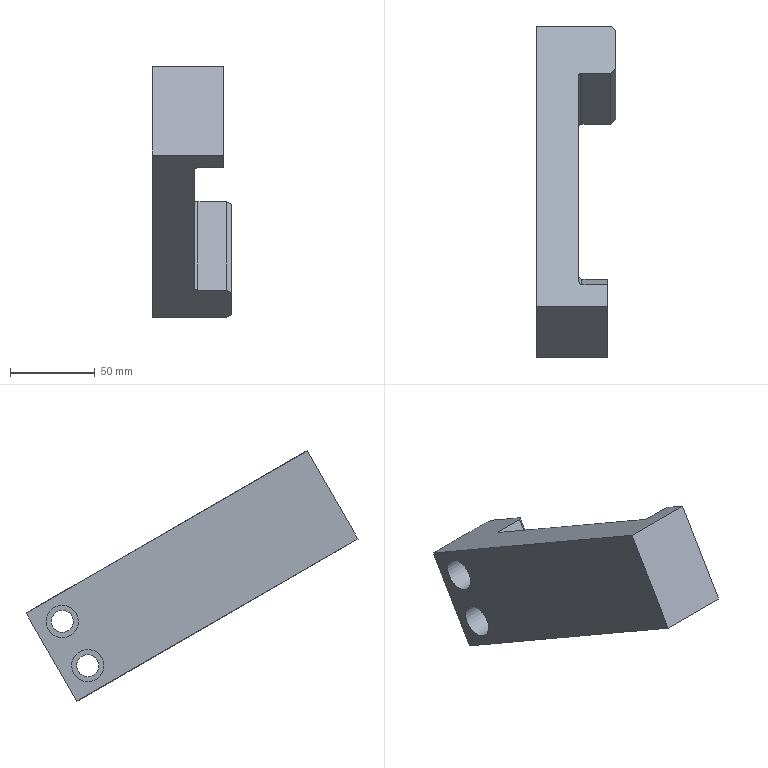Part | NX | features MAIN_BODY 2 | 1 solid | 28 faces | box 47 x 195.411 x 147.462 mm | volume 335091 mm3 | plane 16 | cylinder 10 | spline 2 | commonest cylinder face diameters 4 x4 10 x2 13 x2 19 x2
STEP:
#1=CARTESIAN_POINT('',(-607.,713.604,-62.591));
#2=VERTEX_POINT('',#1);
#3=CARTESIAN_POINT('',(-607.,721.831,-67.341));
#4=DIRECTION('',(-1.,0.,0.));
#5=DIRECTION('',(0.,-0.866,0.5));
#6=AXIS2_PLACEMENT_3D('',#3,#4,#5);
#7=CIRCLE('',#6,9.5);
#8=EDGE_CURVE('',#2,#2,#7,.T.);
#9=ORIENTED_EDGE('',*,*,#8,.F.);
#10=EDGE_LOOP('',(#9));
#11=FACE_BOUND('',#10,.T.);
#12=CARTESIAN_POINT('',(-607.,743.188,-62.351));
#13=VERTEX_POINT('',#12);
#14=CARTESIAN_POINT('',(-607.,577.777,33.149));
#15=VERTEX_POINT('',#14);
#16=CARTESIAN_POINT('',(-607.,743.188,-62.351));
#17=DIRECTION('',(0.,-0.866,0.5));
#18=VECTOR('',#17,1000.);
#19=LINE('',#16,#18);
#20=EDGE_CURVE('',#13,#15,#19,.T.);
#21=ORIENTED_EDGE('',*,*,#20,.F.);
#22=CARTESIAN_POINT('',(-607.,713.188,-114.312));
#23=VERTEX_POINT('',#22);
#24=CARTESIAN_POINT('',(-607.,713.188,-114.312));
#25=DIRECTION('',(0.,0.5,0.866));
#26=VECTOR('',#25,1000.);
#27=LINE('',#24,#26);
#28=EDGE_CURVE('',#23,#13,#27,.T.);
#29=ORIENTED_EDGE('',*,*,#28,.F.);
#30=CARTESIAN_POINT('',(-607.,547.777,-18.812));
#31=VERTEX_POINT('',#30);
#32=CARTESIAN_POINT('',(-607.,547.777,-18.812));
#33=DIRECTION('',(0.,0.866,-0.5));
#34=VECTOR('',#33,1000.);
#35=LINE('',#32,#34);
#36=EDGE_CURVE('',#31,#23,#35,.T.);
#37=ORIENTED_EDGE('',*,*,#36,.F.);
#38=CARTESIAN_POINT('',(-607.,577.777,33.149));
#39=DIRECTION('',(0.,-0.5,-0.866));
#40=VECTOR('',#39,1000.);
#41=LINE('',#38,#40);
#42=EDGE_CURVE('',#15,#31,#41,.T.);
#43=ORIENTED_EDGE('',*,*,#42,.F.);
#44=EDGE_LOOP('',(#21,#29,#37,#43));
#45=FACE_BOUND('',#44,.T.);
#46=CARTESIAN_POINT('',(-607.,698.604,-88.572));
#47=VERTEX_POINT('',#46);
#48=CARTESIAN_POINT('',(-607.,706.831,-93.322));
#49=DIRECTION('',(-1.,0.,0.));
#50=DIRECTION('',(0.,-0.866,0.5));
#51=AXIS2_PLACEMENT_3D('',#48,#49,#50);
#52=CIRCLE('',#51,9.5);
#53=EDGE_CURVE('',#47,#47,#52,.T.);
#54=ORIENTED_EDGE('',*,*,#53,.F.);
#55=EDGE_LOOP('',(#54));
#56=FACE_BOUND('',#55,.T.);
#57=CARTESIAN_POINT('',(-607.,743.188,-62.351));
#58=DIRECTION('',(-1.,0.,0.));
#59=DIRECTION('',(0.,0.866,-0.5));
#60=AXIS2_PLACEMENT_3D('',#57,#58,#59);
#61=PLANE('',#60);
#62=ADVANCED_FACE('',(#11,#45,#56),#61,.T.);
#63=CARTESIAN_POINT('',(-560.,716.202,-64.091));
#64=VERTEX_POINT('',#63);
#65=CARTESIAN_POINT('',(-560.,721.831,-67.341));
#66=DIRECTION('',(-1.,0.,0.));
#67=DIRECTION('',(0.,-0.866,0.5));
#68=AXIS2_PLACEMENT_3D('',#65,#66,#67);
#69=CIRCLE('',#68,6.5);
#70=EDGE_CURVE('',#64,#64,#69,.T.);
#71=ORIENTED_EDGE('',*,*,#70,.T.);
#72=EDGE_LOOP('',(#71));
#73=FACE_BOUND('',#72,.T.);
#74=CARTESIAN_POINT('',(-560.,688.073,-99.812));
#75=VERTEX_POINT('',#74);
#76=CARTESIAN_POINT('',(-560.,710.589,-112.812));
#77=VERTEX_POINT('',#76);
#78=CARTESIAN_POINT('',(-560.,685.475,-98.312));
#79=DIRECTION('',(0.,0.866,-0.5));
#80=VECTOR('',#79,1000.);
#81=LINE('',#78,#80);
#82=EDGE_CURVE('',#75,#77,#81,.T.);
#83=ORIENTED_EDGE('',*,*,#82,.T.);
#84=CARTESIAN_POINT('',(-560.,740.589,-60.851));
#85=VERTEX_POINT('',#84);
#86=CARTESIAN_POINT('',(-560.,710.589,-112.812));
#87=DIRECTION('',(0.,-0.5,-0.866));
#88=VECTOR('',#87,1000.);
#89=LINE('',#86,#88);
#90=EDGE_CURVE('',#85,#77,#89,.T.);
#91=ORIENTED_EDGE('',*,*,#90,.F.);
#92=CARTESIAN_POINT('',(-560.,718.073,-47.851));
#93=VERTEX_POINT('',#92);
#94=CARTESIAN_POINT('',(-560.,743.188,-62.351));
#95=DIRECTION('',(0.,-0.866,0.5));
#96=VECTOR('',#95,1000.);
#97=LINE('',#94,#96);
#98=EDGE_CURVE('',#85,#93,#97,.T.);
#99=ORIENTED_EDGE('',*,*,#98,.T.);
#100=CARTESIAN_POINT('',(-560.,718.073,-47.851));
#101=DIRECTION('',(0.,0.5,0.866));
#102=VECTOR('',#101,1000.);
#103=LINE('',#100,#102);
#104=EDGE_CURVE('',#75,#93,#103,.T.);
#105=ORIENTED_EDGE('',*,*,#104,.F.);
#106=EDGE_LOOP('',(#83,#91,#99,#105));
#107=FACE_BOUND('',#106,.T.);
#108=CARTESIAN_POINT('',(-560.,701.202,-90.072));
#109=VERTEX_POINT('',#108);
#110=CARTESIAN_POINT('',(-560.,706.831,-93.322));
#111=DIRECTION('',(-1.,0.,0.));
#112=DIRECTION('',(0.,-0.866,0.5));
#113=AXIS2_PLACEMENT_3D('',#110,#111,#112);
#114=CIRCLE('',#113,6.5);
#115=EDGE_CURVE('',#109,#109,#114,.T.);
#116=ORIENTED_EDGE('',*,*,#115,.T.);
#117=EDGE_LOOP('',(#116));
#118=FACE_BOUND('',#117,.T.);
#119=CARTESIAN_POINT('',(-560.,715.475,-46.351));
#120=DIRECTION('',(-1.,0.,0.));
#121=DIRECTION('',(0.,0.866,-0.5));
#122=AXIS2_PLACEMENT_3D('',#119,#120,#121);
#123=PLANE('',#122);
#124=ADVANCED_FACE('',(#73,#107,#118),#123,.F.);
#125=CARTESIAN_POINT('',(-582.,713.743,-45.351));
#126=VERTEX_POINT('',#125);
#127=CARTESIAN_POINT('',(-582.,593.217,24.235));
#128=VERTEX_POINT('',#127);
#129=CARTESIAN_POINT('',(-582.,743.188,-62.351));
#130=DIRECTION('',(0.,-0.866,0.5));
#131=VECTOR('',#130,1000.);
#132=LINE('',#129,#131);
#133=EDGE_CURVE('',#126,#128,#132,.T.);
#134=ORIENTED_EDGE('',*,*,#133,.T.);
#135=CARTESIAN_POINT('',(-582.,596.574,11.707));
#136=VERTEX_POINT('',#135);
#137=CARTESIAN_POINT('',(-582.,592.699,26.167));
#138=DIRECTION('',(0.,0.2588,-0.9659));
#139=VECTOR('',#138,1000.);
#140=LINE('',#137,#139);
#141=EDGE_CURVE('',#136,#128,#140,.F.);
#142=ORIENTED_EDGE('',*,*,#141,.F.);
#143=CARTESIAN_POINT('',(-582.,575.745,-24.369));
#144=VERTEX_POINT('',#143);
#145=CARTESIAN_POINT('',(-582.,596.159,10.989));
#146=DIRECTION('',(0.,-0.5,-0.866));
#147=VECTOR('',#146,1000.);
#148=LINE('',#145,#147);
#149=EDGE_CURVE('',#144,#136,#148,.F.);
#150=ORIENTED_EDGE('',*,*,#149,.F.);
#151=CARTESIAN_POINT('',(-582.,563.217,-27.726));
#152=VERTEX_POINT('',#151);
#153=CARTESIAN_POINT('',(-582.,574.945,-24.584));
#154=DIRECTION('',(0.,-0.9659,-0.2588));
#155=VECTOR('',#154,1000.);
#156=LINE('',#153,#155);
#157=EDGE_CURVE('',#152,#144,#156,.F.);
#158=ORIENTED_EDGE('',*,*,#157,.F.);
#159=CARTESIAN_POINT('',(-582.,683.743,-97.312));
#160=VERTEX_POINT('',#159);
#161=CARTESIAN_POINT('',(-582.,547.777,-18.812));
#162=DIRECTION('',(0.,0.866,-0.5));
#163=VECTOR('',#162,1000.);
#164=LINE('',#161,#163);
#165=EDGE_CURVE('',#152,#160,#164,.T.);
#166=ORIENTED_EDGE('',*,*,#165,.T.);
#167=CARTESIAN_POINT('',(-582.,713.743,-45.351));
#168=DIRECTION('',(0.,-0.5,-0.866));
#169=VECTOR('',#168,1000.);
#170=LINE('',#167,#169);
#171=EDGE_CURVE('',#126,#160,#170,.T.);
#172=ORIENTED_EDGE('',*,*,#171,.F.);
#173=EDGE_LOOP('',(#134,#142,#150,#158,#166,#172));
#174=FACE_BOUND('',#173,.T.);
#175=CARTESIAN_POINT('',(-582.,743.188,-62.351));
#176=DIRECTION('',(-1.,0.,0.));
#177=DIRECTION('',(0.,0.866,-0.5));
#178=AXIS2_PLACEMENT_3D('',#175,#176,#177);
#179=PLANE('',#178);
#180=ADVANCED_FACE('',(#174),#179,.F.);
#181=CARTESIAN_POINT('',(-563.,713.188,-114.312));
#182=VERTEX_POINT('',#181);
#183=CARTESIAN_POINT('',(-582.,713.188,-114.312));
#184=DIRECTION('',(-1.,0.,0.));
#185=VECTOR('',#184,1000.);
#186=LINE('',#183,#185);
#187=EDGE_CURVE('',#182,#23,#186,.T.);
#188=ORIENTED_EDGE('',*,*,#187,.T.);
#189=ORIENTED_EDGE('',*,*,#28,.T.);
#190=CARTESIAN_POINT('',(-563.,743.188,-62.351));
#191=VERTEX_POINT('',#190);
#192=CARTESIAN_POINT('',(-582.,743.188,-62.351));
#193=DIRECTION('',(-1.,0.,0.));
#194=VECTOR('',#193,1000.);
#195=LINE('',#192,#194);
#196=EDGE_CURVE('',#191,#13,#195,.T.);
#197=ORIENTED_EDGE('',*,*,#196,.F.);
#198=CARTESIAN_POINT('',(-563.,743.188,-62.351));
#199=DIRECTION('',(0.,0.5,0.866));
#200=VECTOR('',#199,1000.);
#201=LINE('',#198,#200);
#202=EDGE_CURVE('',#182,#191,#201,.T.);
#203=ORIENTED_EDGE('',*,*,#202,.F.);
#204=EDGE_LOOP('',(#188,#189,#197,#203));
#205=FACE_BOUND('',#204,.T.);
#206=CARTESIAN_POINT('',(-582.,713.188,-114.312));
#207=DIRECTION('',(0.,0.866,-0.5));
#208=DIRECTION('',(1.,0.,0.));
#209=AXIS2_PLACEMENT_3D('',#206,#207,#208);
#210=PLANE('',#209);
#211=ADVANCED_FACE('',(#205),#210,.T.);
#212=ORIENTED_EDGE('',*,*,#98,.F.);
#213=CARTESIAN_POINT('',(-572.5,751.415,-67.101));
#214=DIRECTION('',(0.7071,-0.6124,0.3536));
#215=VECTOR('',#214,1000.);
#216=LINE('',#213,#215);
#217=EDGE_CURVE('',#191,#85,#216,.T.);
#218=ORIENTED_EDGE('',*,*,#217,.F.);
#219=ORIENTED_EDGE('',*,*,#196,.T.);
#220=ORIENTED_EDGE('',*,*,#20,.T.);
#221=CARTESIAN_POINT('',(-565.,577.777,33.149));
#222=VERTEX_POINT('',#221);
#223=CARTESIAN_POINT('',(-582.,577.777,33.149));
#224=DIRECTION('',(-1.,0.,0.));
#225=VECTOR('',#224,1000.);
#226=LINE('',#223,#225);
#227=EDGE_CURVE('',#222,#15,#226,.T.);
#228=ORIENTED_EDGE('',*,*,#227,.F.);
#229=CARTESIAN_POINT('',(-565.,590.767,25.649));
#230=VERTEX_POINT('',#229);
#231=CARTESIAN_POINT('',(-565.,743.188,-62.351));
#232=DIRECTION('',(0.,-0.866,0.5));
#233=VECTOR('',#232,1000.);
#234=LINE('',#231,#233);
#235=EDGE_CURVE('',#230,#222,#234,.T.);
#236=ORIENTED_EDGE('',*,*,#235,.F.);
#237=CARTESIAN_POINT('',(-580.,590.767,25.649));
#238=VERTEX_POINT('',#237);
#239=CARTESIAN_POINT('',(-565.,590.767,25.649));
#240=DIRECTION('',(-1.,0.,0.));
#241=VECTOR('',#240,1000.);
#242=LINE('',#239,#241);
#243=EDGE_CURVE('',#230,#238,#242,.T.);
#244=ORIENTED_EDGE('',*,*,#243,.T.);
#245=CARTESIAN_POINT('',(-580.,593.217,24.235));
#246=DIRECTION('',(0.,-0.5,-0.866));
#247=DIRECTION('',(0.,-0.866,0.5));
#248=AXIS2_PLACEMENT_3D('',#245,#246,#247);
#249=ELLIPSE('',#248,2.828,2.);
#250=EDGE_CURVE('',#128,#238,#249,.F.);
#251=ORIENTED_EDGE('',*,*,#250,.F.);
#252=ORIENTED_EDGE('',*,*,#133,.F.);
#253=CARTESIAN_POINT('',(-580.,715.475,-46.351));
#254=VERTEX_POINT('',#253);
#255=CARTESIAN_POINT('',(-580.,713.743,-45.351));
#256=DIRECTION('',(0.,-0.5,-0.866));
#257=DIRECTION('',(1.,0.,0.));
#258=AXIS2_PLACEMENT_3D('',#255,#256,#257);
#259=CIRCLE('',#258,2.);
#260=EDGE_CURVE('',#254,#126,#259,.F.);
#261=ORIENTED_EDGE('',*,*,#260,.F.);
#262=CARTESIAN_POINT('',(-563.,715.475,-46.351));
#263=VERTEX_POINT('',#262);
#264=CARTESIAN_POINT('',(-560.,715.475,-46.351));
#265=DIRECTION('',(-1.,0.,0.));
#266=VECTOR('',#265,1000.);
#267=LINE('',#264,#266);
#268=EDGE_CURVE('',#263,#254,#267,.T.);
#269=ORIENTED_EDGE('',*,*,#268,.F.);
#270=CARTESIAN_POINT('',(-556.5,721.104,-49.601));
#271=DIRECTION('',(-0.7071,-0.6124,0.3536));
#272=VECTOR('',#271,1000.);
#273=LINE('',#270,#272);
#274=EDGE_CURVE('',#93,#263,#273,.T.);
#275=ORIENTED_EDGE('',*,*,#274,.F.);
#276=EDGE_LOOP('',(#212,#218,#219,#220,#228,#236,#244,#251,#252,#261,#269,#275));
#277=FACE_BOUND('',#276,.T.);
#278=CARTESIAN_POINT('',(-582.,743.188,-62.351));
#279=DIRECTION('',(0.,0.5,0.866));
#280=DIRECTION('',(1.,0.,0.));
#281=AXIS2_PLACEMENT_3D('',#278,#279,#280);
#282=PLANE('',#281);
#283=ADVANCED_FACE('',(#277),#282,.T.);
#284=ORIENTED_EDGE('',*,*,#42,.T.);
#285=CARTESIAN_POINT('',(-565.,547.777,-18.812));
#286=VERTEX_POINT('',#285);
#287=CARTESIAN_POINT('',(-582.,547.777,-18.812));
#288=DIRECTION('',(-1.,0.,0.));
#289=VECTOR('',#288,1000.);
#290=LINE('',#287,#289);
#291=EDGE_CURVE('',#286,#31,#290,.T.);
#292=ORIENTED_EDGE('',*,*,#291,.F.);
#293=CARTESIAN_POINT('',(-565.,577.777,33.149));
#294=DIRECTION('',(0.,-0.5,-0.866));
#295=VECTOR('',#294,1000.);
#296=LINE('',#293,#295);
#297=EDGE_CURVE('',#222,#286,#296,.T.);
#298=ORIENTED_EDGE('',*,*,#297,.F.);
#299=ORIENTED_EDGE('',*,*,#227,.T.);
#300=EDGE_LOOP('',(#284,#292,#298,#299));
#301=FACE_BOUND('',#300,.T.);
#302=CARTESIAN_POINT('',(-582.,577.777,33.149));
#303=DIRECTION('',(0.,-0.866,0.5));
#304=DIRECTION('',(0.,0.5,0.866));
#305=AXIS2_PLACEMENT_3D('',#302,#303,#304);
#306=PLANE('',#305);
#307=ADVANCED_FACE('',(#301),#306,.T.);
#308=CARTESIAN_POINT('',(-563.,685.475,-98.312));
#309=VERTEX_POINT('',#308);
#310=CARTESIAN_POINT('',(-580.,685.475,-98.312));
#311=VERTEX_POINT('',#310);
#312=CARTESIAN_POINT('',(-560.,685.475,-98.312));
#313=DIRECTION('',(-1.,0.,0.));
#314=VECTOR('',#313,1000.);
#315=LINE('',#312,#314);
#316=EDGE_CURVE('',#309,#311,#315,.T.);
#317=ORIENTED_EDGE('',*,*,#316,.T.);
#318=CARTESIAN_POINT('',(-580.,683.743,-97.312));
#319=DIRECTION('',(0.,0.5,0.866));
#320=DIRECTION('',(0.,-0.866,0.5));
#321=AXIS2_PLACEMENT_3D('',#318,#319,#320);
#322=CIRCLE('',#321,2.);
#323=EDGE_CURVE('',#160,#311,#322,.F.);
#324=ORIENTED_EDGE('',*,*,#323,.F.);
#325=ORIENTED_EDGE('',*,*,#165,.F.);
#326=CARTESIAN_POINT('',(-580.,560.767,-26.312));
#327=VERTEX_POINT('',#326);
#328=CARTESIAN_POINT('',(-580.,563.217,-27.726));
#329=DIRECTION('',(0.,0.5,0.866));
#330=DIRECTION('',(0.,0.866,-0.5));
#331=AXIS2_PLACEMENT_3D('',#328,#329,#330);
#332=ELLIPSE('',#331,2.828,2.);
#333=EDGE_CURVE('',#327,#152,#332,.F.);
#334=ORIENTED_EDGE('',*,*,#333,.F.);
#335=CARTESIAN_POINT('',(-565.,560.767,-26.312));
#336=VERTEX_POINT('',#335);
#337=CARTESIAN_POINT('',(-565.,560.767,-26.312));
#338=DIRECTION('',(-1.,0.,0.));
#339=VECTOR('',#338,1000.);
#340=LINE('',#337,#339);
#341=EDGE_CURVE('',#336,#327,#340,.T.);
#342=ORIENTED_EDGE('',*,*,#341,.F.);
#343=CARTESIAN_POINT('',(-565.,547.777,-18.812));
#344=DIRECTION('',(0.,0.866,-0.5));
#345=VECTOR('',#344,1000.);
#346=LINE('',#343,#345);
#347=EDGE_CURVE('',#286,#336,#346,.T.);
#348=ORIENTED_EDGE('',*,*,#347,.F.);
#349=ORIENTED_EDGE('',*,*,#291,.T.);
#350=ORIENTED_EDGE('',*,*,#36,.T.);
#351=ORIENTED_EDGE('',*,*,#187,.F.);
#352=CARTESIAN_POINT('',(-477.,638.709,-71.312));
#353=DIRECTION('',(-0.7071,0.6124,-0.3536));
#354=VECTOR('',#353,1000.);
#355=LINE('',#352,#354);
#356=EDGE_CURVE('',#77,#182,#355,.T.);
#357=ORIENTED_EDGE('',*,*,#356,.F.);
#358=ORIENTED_EDGE('',*,*,#82,.F.);
#359=CARTESIAN_POINT('',(-652.,608.398,-53.812));
#360=DIRECTION('',(0.7071,0.6124,-0.3536));
#361=VECTOR('',#360,1000.);
#362=LINE('',#359,#361);
#363=EDGE_CURVE('',#309,#75,#362,.T.);
#364=ORIENTED_EDGE('',*,*,#363,.F.);
#365=EDGE_LOOP('',(#317,#324,#325,#334,#342,#348,#349,#350,#351,#357,#358,#364));
#366=FACE_BOUND('',#365,.T.);
#367=CARTESIAN_POINT('',(-582.,547.777,-18.812));
#368=DIRECTION('',(0.,-0.5,-0.866));
#369=DIRECTION('',(0.,-0.866,0.5));
#370=AXIS2_PLACEMENT_3D('',#367,#368,#369);
#371=PLANE('',#370);
#372=ADVANCED_FACE('',(#366),#371,.T.);
#373=ORIENTED_EDGE('',*,*,#316,.F.);
#374=CARTESIAN_POINT('',(-563.,685.475,-98.312));
#375=DIRECTION('',(0.,-0.5,-0.866));
#376=VECTOR('',#375,1000.);
#377=LINE('',#374,#376);
#378=EDGE_CURVE('',#263,#309,#377,.T.);
#379=ORIENTED_EDGE('',*,*,#378,.F.);
#380=ORIENTED_EDGE('',*,*,#268,.T.);
#381=CARTESIAN_POINT('',(-580.,715.475,-46.351));
#382=DIRECTION('',(0.,-0.5,-0.866));
#383=VECTOR('',#382,1000.);
#384=LINE('',#381,#383);
#385=EDGE_CURVE('',#311,#254,#384,.F.);
#386=ORIENTED_EDGE('',*,*,#385,.F.);
#387=EDGE_LOOP('',(#373,#379,#380,#386));
#388=FACE_BOUND('',#387,.T.);
#389=CARTESIAN_POINT('',(-560.,715.475,-46.351));
#390=DIRECTION('',(0.,-0.866,0.5));
#391=DIRECTION('',(-1.,0.,0.));
#392=AXIS2_PLACEMENT_3D('',#389,#390,#391);
#393=PLANE('',#392);
#394=ADVANCED_FACE('',(#388),#393,.T.);
#395=CARTESIAN_POINT('',(-565.,593.392,10.196));
#396=VERTEX_POINT('',#395);
#397=CARTESIAN_POINT('',(-565.,575.463,-20.858));
#398=VERTEX_POINT('',#397);
#399=CARTESIAN_POINT('',(-565.,594.427,11.989));
#400=DIRECTION('',(0.,-0.5,-0.866));
#401=VECTOR('',#400,1000.);
#402=LINE('',#399,#401);
#403=EDGE_CURVE('',#396,#398,#402,.T.);
#404=ORIENTED_EDGE('',*,*,#403,.T.);
#405=CARTESIAN_POINT('',(-580.,575.463,-20.858));
#406=VERTEX_POINT('',#405);
#407=CARTESIAN_POINT('',(-565.,575.463,-20.858));
#408=DIRECTION('',(-1.,0.,0.));
#409=VECTOR('',#408,1000.);
#410=LINE('',#407,#409);
#411=EDGE_CURVE('',#406,#398,#410,.F.);
#412=ORIENTED_EDGE('',*,*,#411,.F.);
#413=CARTESIAN_POINT('',(-580.,593.392,10.196));
#414=VERTEX_POINT('',#413);
#415=CARTESIAN_POINT('',(-580.,574.427,-22.652));
#416=DIRECTION('',(0.,-0.5,-0.866));
#417=VECTOR('',#416,1000.);
#418=LINE('',#415,#417);
#419=EDGE_CURVE('',#414,#406,#418,.T.);
#420=ORIENTED_EDGE('',*,*,#419,.F.);
#421=CARTESIAN_POINT('',(-565.,593.392,10.196));
#422=DIRECTION('',(-1.,0.,0.));
#423=VECTOR('',#422,1000.);
#424=LINE('',#421,#423);
#425=EDGE_CURVE('',#396,#414,#424,.T.);
#426=ORIENTED_EDGE('',*,*,#425,.F.);
#427=EDGE_LOOP('',(#404,#412,#420,#426));
#428=FACE_BOUND('',#427,.T.);
#429=CARTESIAN_POINT('',(-565.,594.427,11.989));
#430=DIRECTION('',(0.,-0.866,0.5));
#431=DIRECTION('',(0.,0.5,0.866));
#432=AXIS2_PLACEMENT_3D('',#429,#430,#431);
#433=PLANE('',#432);
#434=ADVANCED_FACE('',(#428),#433,.F.);
#435=CARTESIAN_POINT('',(-580.,593.891,13.99));
#436=VERTEX_POINT('',#435);
#437=CARTESIAN_POINT('',(-580.,594.427,11.989));
#438=DIRECTION('',(0.,0.2588,-0.9659));
#439=VECTOR('',#438,1000.);
#440=LINE('',#437,#439);
#441=EDGE_CURVE('',#238,#436,#440,.T.);
#442=ORIENTED_EDGE('',*,*,#441,.F.);
#443=ORIENTED_EDGE('',*,*,#243,.F.);
#444=CARTESIAN_POINT('',(-565.,593.891,13.99));
#445=VERTEX_POINT('',#444);
#446=CARTESIAN_POINT('',(-565.,590.767,25.649));
#447=DIRECTION('',(0.,0.2588,-0.9659));
#448=VECTOR('',#447,1000.);
#449=LINE('',#446,#448);
#450=EDGE_CURVE('',#230,#445,#449,.T.);
#451=ORIENTED_EDGE('',*,*,#450,.T.);
#452=CARTESIAN_POINT('',(-565.,593.891,13.99));
#453=DIRECTION('',(-1.,0.,0.));
#454=VECTOR('',#453,1000.);
#455=LINE('',#452,#454);
#456=EDGE_CURVE('',#436,#445,#455,.F.);
#457=ORIENTED_EDGE('',*,*,#456,.F.);
#458=EDGE_LOOP('',(#442,#443,#451,#457));
#459=FACE_BOUND('',#458,.T.);
#460=CARTESIAN_POINT('',(-565.,590.767,25.649));
#461=DIRECTION('',(0.,-0.9659,-0.2588));
#462=DIRECTION('',(0.,-0.2588,0.9659));
#463=AXIS2_PLACEMENT_3D('',#460,#461,#462);
#464=PLANE('',#463);
#465=ADVANCED_FACE('',(#459),#464,.F.);
#466=CARTESIAN_POINT('',(-565.,572.427,-23.188));
#467=VERTEX_POINT('',#466);
#468=CARTESIAN_POINT('',(-565.,574.427,-22.652));
#469=DIRECTION('',(0.,-0.9659,-0.2588));
#470=VECTOR('',#469,1000.);
#471=LINE('',#468,#470);
#472=EDGE_CURVE('',#467,#336,#471,.T.);
#473=ORIENTED_EDGE('',*,*,#472,.T.);
#474=ORIENTED_EDGE('',*,*,#341,.T.);
#475=CARTESIAN_POINT('',(-580.,572.427,-23.188));
#476=VERTEX_POINT('',#475);
#477=CARTESIAN_POINT('',(-580.,560.767,-26.312));
#478=DIRECTION('',(0.,-0.9659,-0.2588));
#479=VECTOR('',#478,1000.);
#480=LINE('',#477,#479);
#481=EDGE_CURVE('',#476,#327,#480,.T.);
#482=ORIENTED_EDGE('',*,*,#481,.F.);
#483=CARTESIAN_POINT('',(-565.,572.427,-23.188));
#484=DIRECTION('',(-1.,0.,0.));
#485=VECTOR('',#484,1000.);
#486=LINE('',#483,#485);
#487=EDGE_CURVE('',#467,#476,#486,.T.);
#488=ORIENTED_EDGE('',*,*,#487,.F.);
#489=EDGE_LOOP('',(#473,#474,#482,#488));
#490=FACE_BOUND('',#489,.T.);
#491=CARTESIAN_POINT('',(-565.,574.427,-22.652));
#492=DIRECTION('',(0.,-0.2588,0.9659));
#493=DIRECTION('',(0.,0.9659,0.2588));
#494=AXIS2_PLACEMENT_3D('',#491,#492,#493);
#495=PLANE('',#494);
#496=ADVANCED_FACE('',(#490),#495,.F.);
#497=ORIENTED_EDGE('',*,*,#450,.F.);
#498=ORIENTED_EDGE('',*,*,#235,.T.);
#499=ORIENTED_EDGE('',*,*,#297,.T.);
#500=ORIENTED_EDGE('',*,*,#347,.T.);
#501=ORIENTED_EDGE('',*,*,#472,.F.);
#502=CARTESIAN_POINT('',(-565.,571.133,-18.358));
#503=DIRECTION('',(1.,0.,0.));
#504=DIRECTION('',(0.,0.866,-0.5));
#505=AXIS2_PLACEMENT_3D('',#502,#503,#504);
#506=CIRCLE('',#505,5.);
#507=EDGE_CURVE('',#398,#467,#506,.F.);
#508=ORIENTED_EDGE('',*,*,#507,.F.);
#509=ORIENTED_EDGE('',*,*,#403,.F.);
#510=CARTESIAN_POINT('',(-565.,589.062,12.696));
#511=DIRECTION('',(1.,0.,0.));
#512=DIRECTION('',(0.,0.866,-0.5));
#513=AXIS2_PLACEMENT_3D('',#510,#511,#512);
#514=CIRCLE('',#513,5.);
#515=EDGE_CURVE('',#445,#396,#514,.F.);
#516=ORIENTED_EDGE('',*,*,#515,.F.);
#517=EDGE_LOOP('',(#497,#498,#499,#500,#501,#508,#509,#516));
#518=FACE_BOUND('',#517,.T.);
#519=CARTESIAN_POINT('',(-565.,599.727,-14.165));
#520=DIRECTION('',(-1.,0.,0.));
#521=DIRECTION('',(0.,0.866,-0.5));
#522=AXIS2_PLACEMENT_3D('',#519,#520,#521);
#523=PLANE('',#522);
#524=ADVANCED_FACE('',(#518),#523,.F.);
#525=CARTESIAN_POINT('',(-592.,716.202,-64.091));
#526=VERTEX_POINT('',#525);
#527=CARTESIAN_POINT('',(-592.,721.831,-67.341));
#528=DIRECTION('',(-1.,0.,0.));
#529=DIRECTION('',(0.,-0.866,0.5));
#530=AXIS2_PLACEMENT_3D('',#527,#528,#529);
#531=CIRCLE('',#530,6.5);
#532=EDGE_CURVE('',#526,#526,#531,.T.);
#533=ORIENTED_EDGE('',*,*,#532,.T.);
#534=EDGE_LOOP('',(#533));
#535=FACE_BOUND('',#534,.T.);
#536=ORIENTED_EDGE('',*,*,#70,.F.);
#537=EDGE_LOOP('',(#536));
#538=FACE_BOUND('',#537,.T.);
#539=CARTESIAN_POINT('',(-560.,721.831,-67.341));
#540=DIRECTION('',(-1.,0.,0.));
#541=DIRECTION('',(0.,0.866,-0.5));
#542=AXIS2_PLACEMENT_3D('',#539,#540,#541);
#543=CYLINDRICAL_SURFACE('',#542,6.5);
#544=ADVANCED_FACE('',(#535,#538),#543,.F.);
#545=CARTESIAN_POINT('',(-592.,701.202,-90.072));
#546=VERTEX_POINT('',#545);
#547=CARTESIAN_POINT('',(-592.,706.831,-93.322));
#548=DIRECTION('',(-1.,0.,0.));
#549=DIRECTION('',(0.,-0.866,0.5));
#550=AXIS2_PLACEMENT_3D('',#547,#548,#549);
#551=CIRCLE('',#550,6.5);
#552=EDGE_CURVE('',#546,#546,#551,.T.);
#553=ORIENTED_EDGE('',*,*,#552,.T.);
#554=EDGE_LOOP('',(#553));
#555=FACE_BOUND('',#554,.T.);
#556=ORIENTED_EDGE('',*,*,#115,.F.);
#557=EDGE_LOOP('',(#556));
#558=FACE_BOUND('',#557,.T.);
#559=CARTESIAN_POINT('',(-560.,706.831,-93.322));
#560=DIRECTION('',(-1.,0.,0.));
#561=DIRECTION('',(0.,0.866,-0.5));
#562=AXIS2_PLACEMENT_3D('',#559,#560,#561);
#563=CYLINDRICAL_SURFACE('',#562,6.5);
#564=ADVANCED_FACE('',(#555,#558),#563,.F.);
#565=CARTESIAN_POINT('',(-592.,713.604,-62.591));
#566=VERTEX_POINT('',#565);
#567=CARTESIAN_POINT('',(-592.,721.831,-67.341));
#568=DIRECTION('',(-1.,0.,0.));
#569=DIRECTION('',(0.,-0.866,0.5));
#570=AXIS2_PLACEMENT_3D('',#567,#568,#569);
#571=CIRCLE('',#570,9.5);
#572=EDGE_CURVE('',#566,#566,#571,.T.);
#573=ORIENTED_EDGE('',*,*,#572,.F.);
#574=EDGE_LOOP('',(#573));
#575=FACE_BOUND('',#574,.T.);
#576=ORIENTED_EDGE('',*,*,#8,.T.);
#577=EDGE_LOOP('',(#576));
#578=FACE_BOUND('',#577,.T.);
#579=CARTESIAN_POINT('',(-592.,721.831,-67.341));
#580=DIRECTION('',(-1.,0.,0.));
#581=DIRECTION('',(0.,0.866,-0.5));
#582=AXIS2_PLACEMENT_3D('',#579,#580,#581);
#583=CYLINDRICAL_SURFACE('',#582,9.5);
#584=ADVANCED_FACE('',(#575,#578),#583,.F.);
#585=ORIENTED_EDGE('',*,*,#532,.F.);
#586=EDGE_LOOP('',(#585));
#587=FACE_BOUND('',#586,.T.);
#588=ORIENTED_EDGE('',*,*,#572,.T.);
#589=EDGE_LOOP('',(#588));
#590=FACE_BOUND('',#589,.T.);
#591=CARTESIAN_POINT('',(-592.,721.831,-67.341));
#592=DIRECTION('',(1.,0.,0.));
#593=DIRECTION('',(0.,-0.866,0.5));
#594=AXIS2_PLACEMENT_3D('',#591,#592,#593);
#595=PLANE('',#594);
#596=ADVANCED_FACE('',(#587,#590),#595,.F.);
#597=CARTESIAN_POINT('',(-592.,698.604,-88.572));
#598=VERTEX_POINT('',#597);
#599=CARTESIAN_POINT('',(-592.,706.831,-93.322));
#600=DIRECTION('',(-1.,0.,0.));
#601=DIRECTION('',(0.,-0.866,0.5));
#602=AXIS2_PLACEMENT_3D('',#599,#600,#601);
#603=CIRCLE('',#602,9.5);
#604=EDGE_CURVE('',#598,#598,#603,.T.);
#605=ORIENTED_EDGE('',*,*,#604,.F.);
#606=EDGE_LOOP('',(#605));
#607=FACE_BOUND('',#606,.T.);
#608=ORIENTED_EDGE('',*,*,#53,.T.);
#609=EDGE_LOOP('',(#608));
#610=FACE_BOUND('',#609,.T.);
#611=CARTESIAN_POINT('',(-592.,706.831,-93.322));
#612=DIRECTION('',(-1.,0.,0.));
#613=DIRECTION('',(0.,0.866,-0.5));
#614=AXIS2_PLACEMENT_3D('',#611,#612,#613);
#615=CYLINDRICAL_SURFACE('',#614,9.5);
#616=ADVANCED_FACE('',(#607,#610),#615,.F.);
#617=ORIENTED_EDGE('',*,*,#552,.F.);
#618=EDGE_LOOP('',(#617));
#619=FACE_BOUND('',#618,.T.);
#620=ORIENTED_EDGE('',*,*,#604,.T.);
#621=EDGE_LOOP('',(#620));
#622=FACE_BOUND('',#621,.T.);
#623=CARTESIAN_POINT('',(-592.,706.831,-93.322));
#624=DIRECTION('',(1.,0.,0.));
#625=DIRECTION('',(0.,-0.866,0.5));
#626=AXIS2_PLACEMENT_3D('',#623,#624,#625);
#627=PLANE('',#626);
#628=ADVANCED_FACE('',(#619,#622),#627,.F.);
#629=ORIENTED_EDGE('',*,*,#481,.T.);
#630=ORIENTED_EDGE('',*,*,#333,.T.);
#631=ORIENTED_EDGE('',*,*,#157,.T.);
#632=CARTESIAN_POINT('',(-580.,575.745,-24.369));
#633=DIRECTION('',(0.,0.3354,0.9421));
#634=DIRECTION('',(0.,0.9421,-0.3354));
#635=AXIS2_PLACEMENT_3D('',#632,#633,#634);
#636=ELLIPSE('',#635,3.522,2.);
#637=EDGE_CURVE('',#476,#144,#636,.F.);
#638=ORIENTED_EDGE('',*,*,#637,.F.);
#639=EDGE_LOOP('',(#629,#630,#631,#638));
#640=FACE_BOUND('',#639,.T.);
#641=CARTESIAN_POINT('',(-580.,574.945,-24.584));
#642=DIRECTION('',(0.,0.9659,0.2588));
#643=DIRECTION('',(0.,0.2588,-0.9659));
#644=AXIS2_PLACEMENT_3D('',#641,#642,#643);
#645=CYLINDRICAL_SURFACE('',#644,2.);
#646=ADVANCED_FACE('',(#640),#645,.F.);
#647=ORIENTED_EDGE('',*,*,#419,.T.);
#648=CARTESIAN_POINT('',(-580.,575.745,-24.369));
#649=DIRECTION('',(0.,0.9968,0.08015));
#650=DIRECTION('',(0.,0.08015,-0.9968));
#651=AXIS2_PLACEMENT_3D('',#648,#649,#650);
#652=ELLIPSE('',#651,3.522,2.);
#653=EDGE_CURVE('',#144,#406,#652,.T.);
#654=ORIENTED_EDGE('',*,*,#653,.F.);
#655=ORIENTED_EDGE('',*,*,#149,.T.);
#656=CARTESIAN_POINT('',(-580.,596.574,11.707));
#657=DIRECTION('',(0.,-0.429,0.9033));
#658=DIRECTION('',(0.,0.9033,0.429));
#659=AXIS2_PLACEMENT_3D('',#656,#657,#658);
#660=ELLIPSE('',#659,3.522,2.);
#661=EDGE_CURVE('',#414,#136,#660,.F.);
#662=ORIENTED_EDGE('',*,*,#661,.F.);
#663=EDGE_LOOP('',(#647,#654,#655,#662));
#664=FACE_BOUND('',#663,.T.);
#665=CARTESIAN_POINT('',(-580.,596.159,10.989));
#666=DIRECTION('',(0.,0.5,0.866));
#667=DIRECTION('',(0.,0.866,-0.5));
#668=AXIS2_PLACEMENT_3D('',#665,#666,#667);
#669=CYLINDRICAL_SURFACE('',#668,2.);
#670=ADVANCED_FACE('',(#664),#669,.F.);
#671=ORIENTED_EDGE('',*,*,#141,.T.);
#672=ORIENTED_EDGE('',*,*,#250,.T.);
#673=ORIENTED_EDGE('',*,*,#441,.T.);
#674=CARTESIAN_POINT('',(-580.,596.574,11.707));
#675=DIRECTION('',(0.,0.6482,0.7615));
#676=DIRECTION('',(0.,0.7615,-0.6482));
#677=AXIS2_PLACEMENT_3D('',#674,#675,#676);
#678=ELLIPSE('',#677,3.522,2.);
#679=EDGE_CURVE('',#136,#436,#678,.T.);
#680=ORIENTED_EDGE('',*,*,#679,.F.);
#681=EDGE_LOOP('',(#671,#672,#673,#680));
#682=FACE_BOUND('',#681,.T.);
#683=CARTESIAN_POINT('',(-580.,592.699,26.167));
#684=DIRECTION('',(0.,-0.2588,0.9659));
#685=DIRECTION('',(0.,0.9659,0.2588));
#686=AXIS2_PLACEMENT_3D('',#683,#684,#685);
#687=CYLINDRICAL_SURFACE('',#686,2.);
#688=ADVANCED_FACE('',(#682),#687,.F.);
#689=ORIENTED_EDGE('',*,*,#679,.T.);
#690=CARTESIAN_POINT('',(-580.,589.062,12.696));
#691=DIRECTION('',(-1.,0.,0.));
#692=DIRECTION('',(0.,-0.866,0.5));
#693=AXIS2_PLACEMENT_3D('',#690,#691,#692);
#694=CIRCLE('',#693,5.);
#695=EDGE_CURVE('',#436,#414,#694,.T.);
#696=ORIENTED_EDGE('',*,*,#695,.T.);
#697=ORIENTED_EDGE('',*,*,#661,.T.);
#698=EDGE_LOOP('',(#689,#696,#697));
#699=FACE_BOUND('',#698,.T.);
#700=CARTESIAN_POINT('',(-580.,593.392,10.196));
#701=CARTESIAN_POINT('',(-580.,594.427,11.989));
#702=CARTESIAN_POINT('',(-580.,593.891,13.99));
#703=CARTESIAN_POINT('',(-580.262,593.392,10.196));
#704=CARTESIAN_POINT('',(-580.15,594.427,11.989));
#705=CARTESIAN_POINT('',(-580.262,593.891,13.99));
#706=CARTESIAN_POINT('',(-580.785,593.557,10.274));
#707=CARTESIAN_POINT('',(-580.45,594.429,11.989));
#708=CARTESIAN_POINT('',(-580.785,594.031,13.871));
#709=CARTESIAN_POINT('',(-581.451,594.265,10.61));
#710=CARTESIAN_POINT('',(-581.127,594.665,11.958));
#711=CARTESIAN_POINT('',(-581.451,594.627,13.363));
#712=CARTESIAN_POINT('',(-581.896,595.324,11.113));
#713=CARTESIAN_POINT('',(-581.809,595.416,11.859));
#714=CARTESIAN_POINT('',(-581.896,595.52,12.603));
#715=CARTESIAN_POINT('',(-582.,596.157,11.509));
#716=CARTESIAN_POINT('',(-582.,596.19,11.757));
#717=CARTESIAN_POINT('',(-582.,596.222,12.005));
#718=CARTESIAN_POINT('',(-582.,596.574,11.707));
#719=CARTESIAN_POINT('',(-582.,596.574,11.707));
#720=CARTESIAN_POINT('',(-582.,596.574,11.707));
#721=(BOUNDED_SURFACE()B_SPLINE_SURFACE(3,2,((#700,#701,#702),(#703,#704,#705),(#706,#707,#708),(#709,#710,#711),(#712,#713,#714),(#715,#716,#717),(#718,#719,#720)),.UNSPECIFIED.,.F.,.F.,.F.)B_SPLINE_SURFACE_WITH_KNOTS((4,1,1,1,4),(3,3),(3.142,3.534,3.927,4.32,4.712),(0.,1.),.UNSPECIFIED.)GEOMETRIC_REPRESENTATION_ITEM()RATIONAL_B_SPLINE_SURFACE(((1.,0.9239,1.),(1.,0.9239,1.),(1.,0.9325,1.),(1.,0.9629,1.),(1.,0.9921,1.),(1.,1.,1.),(1.,1.,1.)))REPRESENTATION_ITEM('')SURFACE());
#722=ADVANCED_FACE('',(#699),#721,.T.);
#723=ORIENTED_EDGE('',*,*,#515,.T.);
#724=ORIENTED_EDGE('',*,*,#425,.T.);
#725=ORIENTED_EDGE('',*,*,#695,.F.);
#726=ORIENTED_EDGE('',*,*,#456,.T.);
#727=EDGE_LOOP('',(#723,#724,#725,#726));
#728=FACE_BOUND('',#727,.T.);
#729=CARTESIAN_POINT('',(-565.,589.062,12.696));
#730=DIRECTION('',(-1.,0.,0.));
#731=DIRECTION('',(0.,0.866,-0.5));
#732=AXIS2_PLACEMENT_3D('',#729,#730,#731);
#733=CYLINDRICAL_SURFACE('',#732,5.);
#734=ADVANCED_FACE('',(#728),#733,.T.);
#735=ORIENTED_EDGE('',*,*,#653,.T.);
#736=CARTESIAN_POINT('',(-580.,571.133,-18.358));
#737=DIRECTION('',(-1.,0.,0.));
#738=DIRECTION('',(0.,-0.866,0.5));
#739=AXIS2_PLACEMENT_3D('',#736,#737,#738);
#740=CIRCLE('',#739,5.);
#741=EDGE_CURVE('',#406,#476,#740,.T.);
#742=ORIENTED_EDGE('',*,*,#741,.T.);
#743=ORIENTED_EDGE('',*,*,#637,.T.);
#744=EDGE_LOOP('',(#735,#742,#743));
#745=FACE_BOUND('',#744,.T.);
#746=CARTESIAN_POINT('',(-580.,572.427,-23.188));
#747=CARTESIAN_POINT('',(-580.,574.427,-22.652));
#748=CARTESIAN_POINT('',(-580.,575.463,-20.858));
#749=CARTESIAN_POINT('',(-580.262,572.427,-23.188));
#750=CARTESIAN_POINT('',(-580.15,574.427,-22.652));
#751=CARTESIAN_POINT('',(-580.262,575.463,-20.858));
#752=CARTESIAN_POINT('',(-580.785,572.6,-23.249));
#753=CARTESIAN_POINT('',(-580.45,574.428,-22.653));
#754=CARTESIAN_POINT('',(-580.785,575.478,-21.041));
#755=CARTESIAN_POINT('',(-581.451,573.338,-23.512));
#756=CARTESIAN_POINT('',(-581.127,574.573,-22.842));
#757=CARTESIAN_POINT('',(-581.451,575.54,-21.822));
#758=CARTESIAN_POINT('',(-581.896,574.442,-23.905));
#759=CARTESIAN_POINT('',(-581.809,575.035,-23.443));
#760=CARTESIAN_POINT('',(-581.896,575.634,-22.991));
#761=CARTESIAN_POINT('',(-582.,575.311,-24.215));
#762=CARTESIAN_POINT('',(-582.,575.509,-24.062));
#763=CARTESIAN_POINT('',(-582.,575.708,-23.91));
#764=CARTESIAN_POINT('',(-582.,575.745,-24.369));
#765=CARTESIAN_POINT('',(-582.,575.745,-24.369));
#766=CARTESIAN_POINT('',(-582.,575.745,-24.369));
#767=(BOUNDED_SURFACE()B_SPLINE_SURFACE(3,2,((#746,#747,#748),(#749,#750,#751),(#752,#753,#754),(#755,#756,#757),(#758,#759,#760),(#761,#762,#763),(#764,#765,#766)),.UNSPECIFIED.,.F.,.F.,.F.)B_SPLINE_SURFACE_WITH_KNOTS((4,1,1,1,4),(3,3),(3.142,3.534,3.927,4.32,4.712),(0.,1.),.UNSPECIFIED.)GEOMETRIC_REPRESENTATION_ITEM()RATIONAL_B_SPLINE_SURFACE(((1.,0.9239,1.),(1.,0.9239,1.),(1.,0.9325,1.),(1.,0.9629,1.),(1.,0.9921,1.),(1.,1.,1.),(1.,1.,1.)))REPRESENTATION_ITEM('')SURFACE());
#768=ADVANCED_FACE('',(#745),#767,.T.);
#769=ORIENTED_EDGE('',*,*,#507,.T.);
#770=ORIENTED_EDGE('',*,*,#487,.T.);
#771=ORIENTED_EDGE('',*,*,#741,.F.);
#772=ORIENTED_EDGE('',*,*,#411,.T.);
#773=EDGE_LOOP('',(#769,#770,#771,#772));
#774=FACE_BOUND('',#773,.T.);
#775=CARTESIAN_POINT('',(-565.,571.133,-18.358));
#776=DIRECTION('',(-1.,0.,0.));
#777=DIRECTION('',(0.,0.866,-0.5));
#778=AXIS2_PLACEMENT_3D('',#775,#776,#777);
#779=CYLINDRICAL_SURFACE('',#778,5.);
#780=ADVANCED_FACE('',(#774),#779,.T.);
#781=ORIENTED_EDGE('',*,*,#274,.T.);
#782=ORIENTED_EDGE('',*,*,#378,.T.);
#783=ORIENTED_EDGE('',*,*,#363,.T.);
#784=ORIENTED_EDGE('',*,*,#104,.T.);
#785=EDGE_LOOP('',(#781,#782,#783,#784));
#786=FACE_BOUND('',#785,.T.);
#787=CARTESIAN_POINT('',(-563.,715.475,-46.351));
#788=DIRECTION('',(0.7071,-0.6124,0.3536));
#789=DIRECTION('',(-0.7071,-0.6124,0.3536));
#790=AXIS2_PLACEMENT_3D('',#787,#788,#789);
#791=PLANE('',#790);
#792=ADVANCED_FACE('',(#786),#791,.T.);
#793=ORIENTED_EDGE('',*,*,#356,.T.);
#794=ORIENTED_EDGE('',*,*,#202,.T.);
#795=ORIENTED_EDGE('',*,*,#217,.T.);
#796=ORIENTED_EDGE('',*,*,#90,.T.);
#797=EDGE_LOOP('',(#793,#794,#795,#796));
#798=FACE_BOUND('',#797,.T.);
#799=CARTESIAN_POINT('',(-563.,713.188,-114.312));
#800=DIRECTION('',(0.7071,0.6124,-0.3536));
#801=DIRECTION('',(0.7071,-0.6124,0.3536));
#802=AXIS2_PLACEMENT_3D('',#799,#800,#801);
#803=PLANE('',#802);
#804=ADVANCED_FACE('',(#798),#803,.T.);
#805=ORIENTED_EDGE('',*,*,#260,.T.);
#806=ORIENTED_EDGE('',*,*,#171,.T.);
#807=ORIENTED_EDGE('',*,*,#323,.T.);
#808=ORIENTED_EDGE('',*,*,#385,.T.);
#809=EDGE_LOOP('',(#805,#806,#807,#808));
#810=FACE_BOUND('',#809,.T.);
#811=CARTESIAN_POINT('',(-580.,713.743,-45.351));
#812=DIRECTION('',(0.,-0.5,-0.866));
#813=DIRECTION('',(-1.,0.,0.));
#814=AXIS2_PLACEMENT_3D('',#811,#812,#813);
#815=CYLINDRICAL_SURFACE('',#814,2.);
#816=ADVANCED_FACE('',(#810),#815,.F.);
#817=CLOSED_SHELL('',(#62,#124,#180,#211,#283,#307,#372,#394,#434,#465,#496,#524,#544,#564,#584,#596,#616,#628,#646,#670,#688,#722,#734,#768,#780,#792,#804,#816));
#818=MANIFOLD_SOLID_BREP('',#817);
#819=(LENGTH_UNIT()NAMED_UNIT(*)SI_UNIT(.MILLI.,.METRE.));
#820=UNCERTAINTY_MEASURE_WITH_UNIT(LENGTH_MEASURE(0.0508),#819,'','');
#821=(NAMED_UNIT(*)PLANE_ANGLE_UNIT()SI_UNIT($,.RADIAN.));
#822=(NAMED_UNIT(*)SI_UNIT($,.STERADIAN.)SOLID_ANGLE_UNIT());
#823=(GEOMETRIC_REPRESENTATION_CONTEXT(3)GLOBAL_UNCERTAINTY_ASSIGNED_CONTEXT((#820))GLOBAL_UNIT_ASSIGNED_CONTEXT((#819,#821,#822))REPRESENTATION_CONTEXT('',''));
#824=ADVANCED_BREP_SHAPE_REPRESENTATION('',(#818),#823);